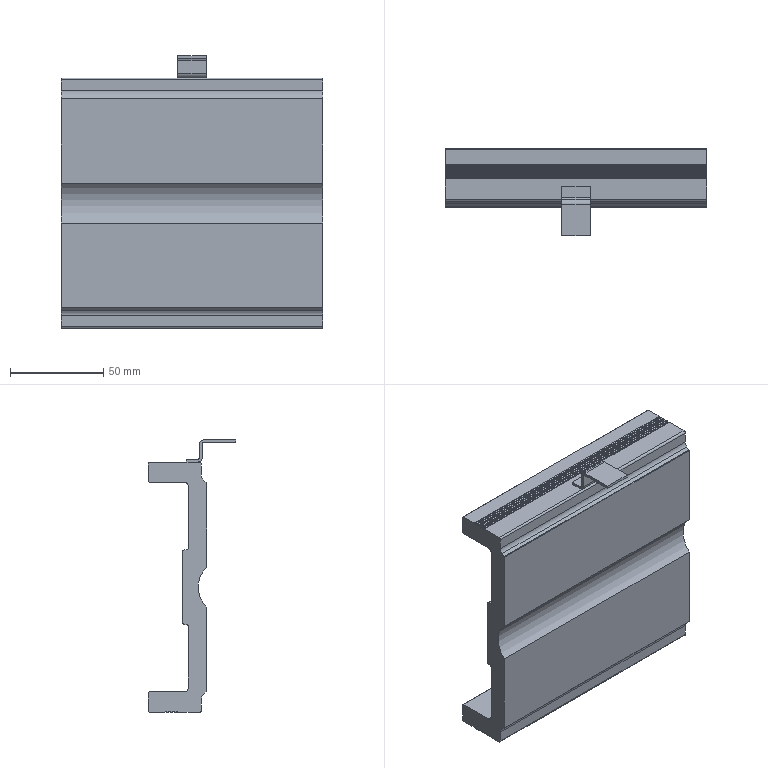Part | SolidWorks | features BaseBody 1 | 1 solid | 131 faces | box 140 x 47 x 146 mm | volume 250263 mm3 | cylinder 63 | plane 52 | cone 16 | commonest cylinder face diameters 1 x28 4.917 x16 2 x8 6 x4 4 x2 5 x2